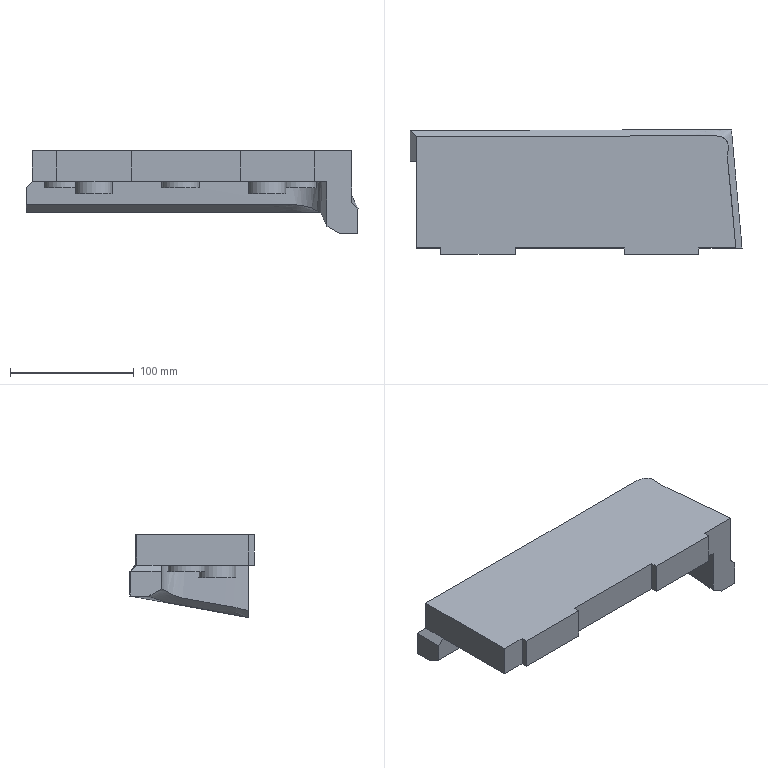Part | NX | features solid 2 | 1 solid | 32 faces | box 268.536 x 100.639 x 67.129 mm | volume 859631 mm3 | plane 20 | spline 7 | cylinder 5 | commonest cylinder face diameters 30 x5